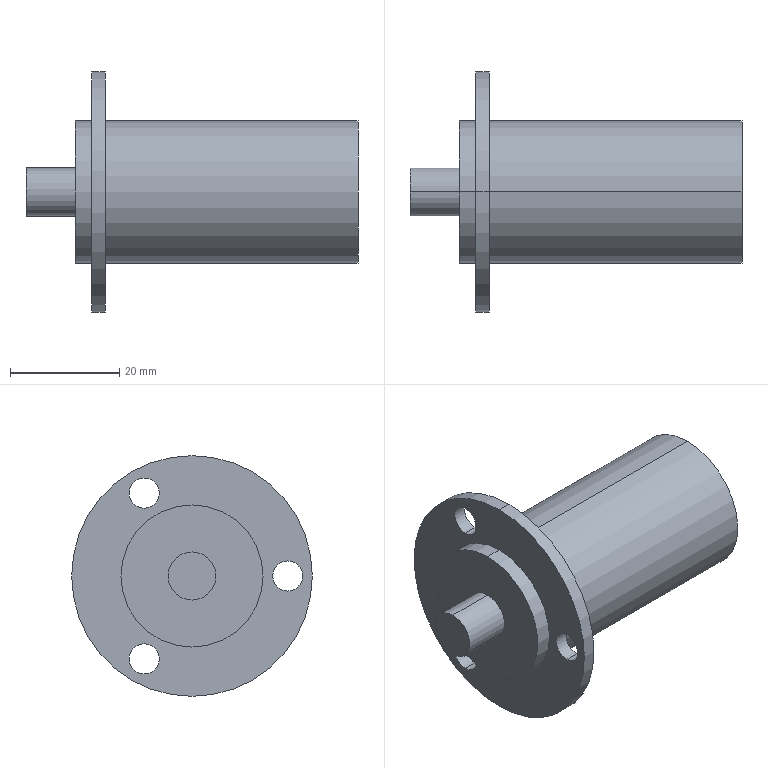Part | STEP file | SRC025-30 rotary joint_SUS304 | 1 solid | 19 faces | box 60.7 x 44 x 44 mm | volume 30292 mm3 | cylinder 14 | plane 5 | commonest cylinder face diameters 5.5 x6 26 x4 8.8 x2 44 x2
STEP:
#1=CARTESIAN_POINT('',(0.,0.,0.));
#2=DIRECTION('',(0.,0.,1.));
#3=DIRECTION('',(1.,0.,0.));
#4=AXIS2_PLACEMENT_3D('',#1,#2,#3);
#5=CARTESIAN_POINT('',(60.7,0.,13.));
#6=VERTEX_POINT('',#5);
#7=CARTESIAN_POINT('',(60.7,0.,-13.));
#8=VERTEX_POINT('',#7);
#9=CARTESIAN_POINT('',(60.7,0.,0.));
#10=DIRECTION('',(-1.,0.,0.));
#11=DIRECTION('',(0.,0.,1.));
#12=AXIS2_PLACEMENT_3D('',#9,#10,#11);
#13=CIRCLE('',#12,13.);
#14=CARTESIAN_POINT('',(60.7,0.,0.));
#15=DIRECTION('',(-1.,0.,0.));
#16=DIRECTION('',(0.,0.,1.));
#17=AXIS2_PLACEMENT_3D('',#14,#15,#16);
#18=CYLINDRICAL_SURFACE('',#17,13.);
#19=CARTESIAN_POINT('',(0.,0.));
#20=DIRECTION('',(1.,0.));
#21=VECTOR('',#20,1.);
#22=LINE('',#19,#21);
#23=(GEOMETRIC_REPRESENTATION_CONTEXT(2)PARAMETRIC_REPRESENTATION_CONTEXT()REPRESENTATION_CONTEXT('',''));
#24=DEFINITIONAL_REPRESENTATION('',(#22),#23);
#25=PCURVE('',#18,#24);
#26=CARTESIAN_POINT('',(60.7,0.,0.));
#27=DIRECTION('',(1.,0.,0.));
#28=DIRECTION('',(0.,0.,-1.));
#29=AXIS2_PLACEMENT_3D('',#26,#27,#28);
#30=PLANE('',#29);
#31=CARTESIAN_POINT('',(-13.,0.));
#32=CARTESIAN_POINT('',(-13.,22.517));
#33=CARTESIAN_POINT('',(6.5,11.258));
#34=CARTESIAN_POINT('',(26.,0.));
#35=CARTESIAN_POINT('',(6.5,-11.258));
#36=CARTESIAN_POINT('',(-13.,-22.517));
#37=CARTESIAN_POINT('',(-13.,0.));
#38=(BOUNDED_CURVE()B_SPLINE_CURVE(2,(#31,#32,#33,#34,#35,#36,#37),.UNSPECIFIED.,.T.,.F.)B_SPLINE_CURVE_WITH_KNOTS((1,2,2,2,2,1),(-2.094,0.,2.094,4.189,6.283,8.378),.UNSPECIFIED.)CURVE()GEOMETRIC_REPRESENTATION_ITEM()RATIONAL_B_SPLINE_CURVE((1.,0.5,1.,0.5,1.,0.5,1.))REPRESENTATION_ITEM(''));
#39=(GEOMETRIC_REPRESENTATION_CONTEXT(2)PARAMETRIC_REPRESENTATION_CONTEXT()REPRESENTATION_CONTEXT('',''));
#40=DEFINITIONAL_REPRESENTATION('',(#38),#39);
#41=PCURVE('',#30,#40);
#42=SURFACE_CURVE('',#13,(#25,#41),.PCURVE_S1.);
#43=EDGE_CURVE('',#6,#8,#42,.T.);
#44=ORIENTED_EDGE('',*,*,#43,.T.);
#45=CARTESIAN_POINT('',(14.5,0.,-13.));
#46=VERTEX_POINT('',#45);
#47=CARTESIAN_POINT('',(60.7,0.,-13.));
#48=DIRECTION('',(-1.,0.,0.));
#49=VECTOR('',#48,1.);
#50=LINE('',#47,#49);
#51=CARTESIAN_POINT('',(3.142,0.));
#52=DIRECTION('',(0.,1.));
#53=VECTOR('',#52,1.);
#54=LINE('',#51,#53);
#55=(GEOMETRIC_REPRESENTATION_CONTEXT(2)PARAMETRIC_REPRESENTATION_CONTEXT()REPRESENTATION_CONTEXT('',''));
#56=DEFINITIONAL_REPRESENTATION('',(#54),#55);
#57=PCURVE('',#18,#56);
#58=CARTESIAN_POINT('',(60.7,0.,0.));
#59=DIRECTION('',(-1.,0.,0.));
#60=DIRECTION('',(0.,0.,1.));
#61=AXIS2_PLACEMENT_3D('',#58,#59,#60);
#62=CYLINDRICAL_SURFACE('',#61,13.);
#63=CARTESIAN_POINT('',(3.142,0.));
#64=DIRECTION('',(0.,1.));
#65=VECTOR('',#64,1.);
#66=LINE('',#63,#65);
#67=(GEOMETRIC_REPRESENTATION_CONTEXT(2)PARAMETRIC_REPRESENTATION_CONTEXT()REPRESENTATION_CONTEXT('',''));
#68=DEFINITIONAL_REPRESENTATION('',(#66),#67);
#69=PCURVE('',#62,#68);
#70=SURFACE_CURVE('',#50,(#57,#69),.PCURVE_S1.);
#71=EDGE_CURVE('',#8,#46,#70,.T.);
#72=ORIENTED_EDGE('',*,*,#71,.T.);
#73=CARTESIAN_POINT('',(14.5,0.,13.));
#74=VERTEX_POINT('',#73);
#75=CARTESIAN_POINT('',(14.5,0.,0.));
#76=DIRECTION('',(1.,0.,0.));
#77=DIRECTION('',(0.,0.,1.));
#78=AXIS2_PLACEMENT_3D('',#75,#76,#77);
#79=CIRCLE('',#78,13.);
#80=CARTESIAN_POINT('',(6.283,46.2));
#81=DIRECTION('',(-1.,0.));
#82=VECTOR('',#81,1.);
#83=LINE('',#80,#82);
#84=(GEOMETRIC_REPRESENTATION_CONTEXT(2)PARAMETRIC_REPRESENTATION_CONTEXT()REPRESENTATION_CONTEXT('',''));
#85=DEFINITIONAL_REPRESENTATION('',(#83),#84);
#86=PCURVE('',#18,#85);
#87=CARTESIAN_POINT('',(14.5,0.,0.));
#88=DIRECTION('',(1.,0.,0.));
#89=DIRECTION('',(0.,0.,-1.));
#90=AXIS2_PLACEMENT_3D('',#87,#88,#89);
#91=PLANE('',#90);
#92=CARTESIAN_POINT('',(0.,0.));
#93=DIRECTION('',(-1.,0.));
#94=AXIS2_PLACEMENT_2D('',#92,#93);
#95=CIRCLE('',#94,13.);
#96=(GEOMETRIC_REPRESENTATION_CONTEXT(2)PARAMETRIC_REPRESENTATION_CONTEXT()REPRESENTATION_CONTEXT('',''));
#97=DEFINITIONAL_REPRESENTATION('',(#95),#96);
#98=PCURVE('',#91,#97);
#99=SURFACE_CURVE('',#79,(#86,#98),.PCURVE_S1.);
#100=EDGE_CURVE('',#46,#74,#99,.T.);
#101=ORIENTED_EDGE('',*,*,#100,.T.);
#102=CARTESIAN_POINT('',(60.7,0.,13.));
#103=DIRECTION('',(-1.,0.,0.));
#104=VECTOR('',#103,1.);
#105=LINE('',#102,#104);
#106=CARTESIAN_POINT('',(0.,0.));
#107=DIRECTION('',(0.,1.));
#108=VECTOR('',#107,1.);
#109=LINE('',#106,#108);
#110=(GEOMETRIC_REPRESENTATION_CONTEXT(2)PARAMETRIC_REPRESENTATION_CONTEXT()REPRESENTATION_CONTEXT('',''));
#111=DEFINITIONAL_REPRESENTATION('',(#109),#110);
#112=PCURVE('',#18,#111);
#113=CARTESIAN_POINT('',(6.283,0.));
#114=DIRECTION('',(0.,1.));
#115=VECTOR('',#114,1.);
#116=LINE('',#113,#115);
#117=(GEOMETRIC_REPRESENTATION_CONTEXT(2)PARAMETRIC_REPRESENTATION_CONTEXT()REPRESENTATION_CONTEXT('',''));
#118=DEFINITIONAL_REPRESENTATION('',(#116),#117);
#119=PCURVE('',#62,#118);
#120=SURFACE_CURVE('',#105,(#112,#119),.PCURVE_S1.);
#121=EDGE_CURVE('',#6,#74,#120,.T.);
#122=ORIENTED_EDGE('',*,*,#121,.F.);
#123=EDGE_LOOP('',(#44,#72,#101,#122));
#124=FACE_BOUND('',#123,.T.);
#125=ADVANCED_FACE('',(#124),#18,.T.);
#126=CARTESIAN_POINT('',(14.5,-17.5,2.75));
#127=VERTEX_POINT('',#126);
#128=CARTESIAN_POINT('',(12.,-17.5,2.75));
#129=VERTEX_POINT('',#128);
#130=CARTESIAN_POINT('',(58.2,-17.5,2.75));
#131=DIRECTION('',(-1.,0.,0.));
#132=VECTOR('',#131,1.);
#133=LINE('',#130,#132);
#134=CARTESIAN_POINT('',(58.2,-17.5,0.));
#135=DIRECTION('',(-1.,0.,0.));
#136=DIRECTION('',(0.,0.,1.));
#137=AXIS2_PLACEMENT_3D('',#134,#135,#136);
#138=CYLINDRICAL_SURFACE('',#137,2.75);
#139=CARTESIAN_POINT('',(6.283,0.));
#140=DIRECTION('',(0.,1.));
#141=VECTOR('',#140,1.);
#142=LINE('',#139,#141);
#143=(GEOMETRIC_REPRESENTATION_CONTEXT(2)PARAMETRIC_REPRESENTATION_CONTEXT()REPRESENTATION_CONTEXT('',''));
#144=DEFINITIONAL_REPRESENTATION('',(#142),#143);
#145=PCURVE('',#138,#144);
#146=CARTESIAN_POINT('',(58.2,-17.5,0.));
#147=DIRECTION('',(-1.,0.,0.));
#148=DIRECTION('',(0.,0.,1.));
#149=AXIS2_PLACEMENT_3D('',#146,#147,#148);
#150=CYLINDRICAL_SURFACE('',#149,2.75);
#151=CARTESIAN_POINT('',(0.,0.));
#152=DIRECTION('',(0.,1.));
#153=VECTOR('',#152,1.);
#154=LINE('',#151,#153);
#155=(GEOMETRIC_REPRESENTATION_CONTEXT(2)PARAMETRIC_REPRESENTATION_CONTEXT()REPRESENTATION_CONTEXT('',''));
#156=DEFINITIONAL_REPRESENTATION('',(#154),#155);
#157=PCURVE('',#150,#156);
#158=SURFACE_CURVE('',#133,(#145,#157),.PCURVE_S1.);
#159=EDGE_CURVE('',#127,#129,#158,.T.);
#160=ORIENTED_EDGE('',*,*,#159,.T.);
#161=CARTESIAN_POINT('',(12.,-17.5,-2.75));
#162=VERTEX_POINT('',#161);
#163=CARTESIAN_POINT('',(12.,-17.5,0.));
#164=DIRECTION('',(1.,0.,0.));
#165=DIRECTION('',(0.,0.,1.));
#166=AXIS2_PLACEMENT_3D('',#163,#164,#165);
#167=CIRCLE('',#166,2.75);
#168=CARTESIAN_POINT('',(6.283,46.2));
#169=DIRECTION('',(-1.,0.));
#170=VECTOR('',#169,1.);
#171=LINE('',#168,#170);
#172=(GEOMETRIC_REPRESENTATION_CONTEXT(2)PARAMETRIC_REPRESENTATION_CONTEXT()REPRESENTATION_CONTEXT('',''));
#173=DEFINITIONAL_REPRESENTATION('',(#171),#172);
#174=PCURVE('',#138,#173);
#175=CARTESIAN_POINT('',(12.,0.,0.));
#176=DIRECTION('',(1.,0.,0.));
#177=DIRECTION('',(0.,0.,-1.));
#178=AXIS2_PLACEMENT_3D('',#175,#176,#177);
#179=PLANE('',#178);
#180=CARTESIAN_POINT('',(0.,-17.5));
#181=DIRECTION('',(-1.,0.));
#182=AXIS2_PLACEMENT_2D('',#180,#181);
#183=CIRCLE('',#182,2.75);
#184=(GEOMETRIC_REPRESENTATION_CONTEXT(2)PARAMETRIC_REPRESENTATION_CONTEXT()REPRESENTATION_CONTEXT('',''));
#185=DEFINITIONAL_REPRESENTATION('',(#183),#184);
#186=PCURVE('',#179,#185);
#187=SURFACE_CURVE('',#167,(#174,#186),.PCURVE_S1.);
#188=EDGE_CURVE('',#129,#162,#187,.T.);
#189=ORIENTED_EDGE('',*,*,#188,.T.);
#190=CARTESIAN_POINT('',(14.5,-17.5,-2.75));
#191=VERTEX_POINT('',#190);
#192=CARTESIAN_POINT('',(58.2,-17.5,-2.75));
#193=DIRECTION('',(-1.,0.,0.));
#194=VECTOR('',#193,1.);
#195=LINE('',#192,#194);
#196=CARTESIAN_POINT('',(3.142,0.));
#197=DIRECTION('',(0.,1.));
#198=VECTOR('',#197,1.);
#199=LINE('',#196,#198);
#200=(GEOMETRIC_REPRESENTATION_CONTEXT(2)PARAMETRIC_REPRESENTATION_CONTEXT()REPRESENTATION_CONTEXT('',''));
#201=DEFINITIONAL_REPRESENTATION('',(#199),#200);
#202=PCURVE('',#138,#201);
#203=CARTESIAN_POINT('',(3.142,0.));
#204=DIRECTION('',(0.,1.));
#205=VECTOR('',#204,1.);
#206=LINE('',#203,#205);
#207=(GEOMETRIC_REPRESENTATION_CONTEXT(2)PARAMETRIC_REPRESENTATION_CONTEXT()REPRESENTATION_CONTEXT('',''));
#208=DEFINITIONAL_REPRESENTATION('',(#206),#207);
#209=PCURVE('',#150,#208);
#210=SURFACE_CURVE('',#195,(#202,#209),.PCURVE_S1.);
#211=EDGE_CURVE('',#191,#162,#210,.T.);
#212=ORIENTED_EDGE('',*,*,#211,.F.);
#213=CARTESIAN_POINT('',(14.5,-17.5,0.));
#214=DIRECTION('',(-1.,0.,0.));
#215=DIRECTION('',(0.,0.,1.));
#216=AXIS2_PLACEMENT_3D('',#213,#214,#215);
#217=CIRCLE('',#216,2.75);
#218=CARTESIAN_POINT('',(0.,43.7));
#219=DIRECTION('',(1.,0.));
#220=VECTOR('',#219,1.);
#221=LINE('',#218,#220);
#222=(GEOMETRIC_REPRESENTATION_CONTEXT(2)PARAMETRIC_REPRESENTATION_CONTEXT()REPRESENTATION_CONTEXT('',''));
#223=DEFINITIONAL_REPRESENTATION('',(#221),#222);
#224=PCURVE('',#138,#223);
#225=CARTESIAN_POINT('',(-2.75,-17.5));
#226=CARTESIAN_POINT('',(-2.75,-12.737));
#227=CARTESIAN_POINT('',(1.375,-15.118));
#228=CARTESIAN_POINT('',(5.5,-17.5));
#229=CARTESIAN_POINT('',(1.375,-19.882));
#230=CARTESIAN_POINT('',(-2.75,-22.263));
#231=CARTESIAN_POINT('',(-2.75,-17.5));
#232=(BOUNDED_CURVE()B_SPLINE_CURVE(2,(#225,#226,#227,#228,#229,#230,#231),.UNSPECIFIED.,.T.,.F.)B_SPLINE_CURVE_WITH_KNOTS((1,2,2,2,2,1),(-2.094,0.,2.094,4.189,6.283,8.378),.UNSPECIFIED.)CURVE()GEOMETRIC_REPRESENTATION_ITEM()RATIONAL_B_SPLINE_CURVE((1.,0.5,1.,0.5,1.,0.5,1.))REPRESENTATION_ITEM(''));
#233=(GEOMETRIC_REPRESENTATION_CONTEXT(2)PARAMETRIC_REPRESENTATION_CONTEXT()REPRESENTATION_CONTEXT('',''));
#234=DEFINITIONAL_REPRESENTATION('',(#232),#233);
#235=PCURVE('',#91,#234);
#236=SURFACE_CURVE('',#217,(#224,#235),.PCURVE_S1.);
#237=EDGE_CURVE('',#191,#127,#236,.T.);
#238=ORIENTED_EDGE('',*,*,#237,.T.);
#239=EDGE_LOOP('',(#160,#189,#212,#238));
#240=FACE_BOUND('',#239,.F.);
#241=ADVANCED_FACE('',(#240),#138,.F.);
#242=CARTESIAN_POINT('',(14.5,8.75,-12.405));
#243=VERTEX_POINT('',#242);
#244=CARTESIAN_POINT('',(12.,8.75,-12.405));
#245=VERTEX_POINT('',#244);
#246=CARTESIAN_POINT('',(58.2,8.75,-12.405));
#247=DIRECTION('',(-1.,0.,0.));
#248=VECTOR('',#247,1.);
#249=LINE('',#246,#248);
#250=CARTESIAN_POINT('',(58.2,8.75,-15.155));
#251=DIRECTION('',(-1.,0.,0.));
#252=DIRECTION('',(0.,0.,1.));
#253=AXIS2_PLACEMENT_3D('',#250,#251,#252);
#254=CYLINDRICAL_SURFACE('',#253,2.75);
#255=CARTESIAN_POINT('',(6.283,0.));
#256=DIRECTION('',(0.,1.));
#257=VECTOR('',#256,1.);
#258=LINE('',#255,#257);
#259=(GEOMETRIC_REPRESENTATION_CONTEXT(2)PARAMETRIC_REPRESENTATION_CONTEXT()REPRESENTATION_CONTEXT('',''));
#260=DEFINITIONAL_REPRESENTATION('',(#258),#259);
#261=PCURVE('',#254,#260);
#262=CARTESIAN_POINT('',(58.2,8.75,-15.155));
#263=DIRECTION('',(-1.,0.,0.));
#264=DIRECTION('',(0.,0.,1.));
#265=AXIS2_PLACEMENT_3D('',#262,#263,#264);
#266=CYLINDRICAL_SURFACE('',#265,2.75);
#267=CARTESIAN_POINT('',(0.,0.));
#268=DIRECTION('',(0.,1.));
#269=VECTOR('',#268,1.);
#270=LINE('',#267,#269);
#271=(GEOMETRIC_REPRESENTATION_CONTEXT(2)PARAMETRIC_REPRESENTATION_CONTEXT()REPRESENTATION_CONTEXT('',''));
#272=DEFINITIONAL_REPRESENTATION('',(#270),#271);
#273=PCURVE('',#266,#272);
#274=SURFACE_CURVE('',#249,(#261,#273),.PCURVE_S1.);
#275=EDGE_CURVE('',#243,#245,#274,.T.);
#276=ORIENTED_EDGE('',*,*,#275,.T.);
#277=CARTESIAN_POINT('',(12.,8.75,-17.905));
#278=VERTEX_POINT('',#277);
#279=CARTESIAN_POINT('',(12.,8.75,-15.155));
#280=DIRECTION('',(1.,0.,0.));
#281=DIRECTION('',(0.,0.,1.));
#282=AXIS2_PLACEMENT_3D('',#279,#280,#281);
#283=CIRCLE('',#282,2.75);
#284=CARTESIAN_POINT('',(6.283,46.2));
#285=DIRECTION('',(-1.,0.));
#286=VECTOR('',#285,1.);
#287=LINE('',#284,#286);
#288=(GEOMETRIC_REPRESENTATION_CONTEXT(2)PARAMETRIC_REPRESENTATION_CONTEXT()REPRESENTATION_CONTEXT('',''));
#289=DEFINITIONAL_REPRESENTATION('',(#287),#288);
#290=PCURVE('',#254,#289);
#291=CARTESIAN_POINT('',(15.155,8.75));
#292=DIRECTION('',(-1.,0.));
#293=AXIS2_PLACEMENT_2D('',#291,#292);
#294=CIRCLE('',#293,2.75);
#295=(GEOMETRIC_REPRESENTATION_CONTEXT(2)PARAMETRIC_REPRESENTATION_CONTEXT()REPRESENTATION_CONTEXT('',''));
#296=DEFINITIONAL_REPRESENTATION('',(#294),#295);
#297=PCURVE('',#179,#296);
#298=SURFACE_CURVE('',#283,(#290,#297),.PCURVE_S1.);
#299=EDGE_CURVE('',#245,#278,#298,.T.);
#300=ORIENTED_EDGE('',*,*,#299,.T.);
#301=CARTESIAN_POINT('',(14.5,8.75,-17.905));
#302=VERTEX_POINT('',#301);
#303=CARTESIAN_POINT('',(58.2,8.75,-17.905));
#304=DIRECTION('',(-1.,0.,0.));
#305=VECTOR('',#304,1.);
#306=LINE('',#303,#305);
#307=CARTESIAN_POINT('',(3.142,0.));
#308=DIRECTION('',(0.,1.));
#309=VECTOR('',#308,1.);
#310=LINE('',#307,#309);
#311=(GEOMETRIC_REPRESENTATION_CONTEXT(2)PARAMETRIC_REPRESENTATION_CONTEXT()REPRESENTATION_CONTEXT('',''));
#312=DEFINITIONAL_REPRESENTATION('',(#310),#311);
#313=PCURVE('',#254,#312);
#314=CARTESIAN_POINT('',(3.142,0.));
#315=DIRECTION('',(0.,1.));
#316=VECTOR('',#315,1.);
#317=LINE('',#314,#316);
#318=(GEOMETRIC_REPRESENTATION_CONTEXT(2)PARAMETRIC_REPRESENTATION_CONTEXT()REPRESENTATION_CONTEXT('',''));
#319=DEFINITIONAL_REPRESENTATION('',(#317),#318);
#320=PCURVE('',#266,#319);
#321=SURFACE_CURVE('',#306,(#313,#320),.PCURVE_S1.);
#322=EDGE_CURVE('',#302,#278,#321,.T.);
#323=ORIENTED_EDGE('',*,*,#322,.F.);
#324=CARTESIAN_POINT('',(14.5,8.75,-15.155));
#325=DIRECTION('',(-1.,0.,0.));
#326=DIRECTION('',(0.,0.,1.));
#327=AXIS2_PLACEMENT_3D('',#324,#325,#326);
#328=CIRCLE('',#327,2.75);
#329=CARTESIAN_POINT('',(0.,43.7));
#330=DIRECTION('',(1.,0.));
#331=VECTOR('',#330,1.);
#332=LINE('',#329,#331);
#333=(GEOMETRIC_REPRESENTATION_CONTEXT(2)PARAMETRIC_REPRESENTATION_CONTEXT()REPRESENTATION_CONTEXT('',''));
#334=DEFINITIONAL_REPRESENTATION('',(#332),#333);
#335=PCURVE('',#254,#334);
#336=CARTESIAN_POINT('',(12.405,8.75));
#337=CARTESIAN_POINT('',(12.405,13.513));
#338=CARTESIAN_POINT('',(16.53,11.132));
#339=CARTESIAN_POINT('',(20.655,8.75));
#340=CARTESIAN_POINT('',(16.53,6.368));
#341=CARTESIAN_POINT('',(12.405,3.987));
#342=CARTESIAN_POINT('',(12.405,8.75));
#343=(BOUNDED_CURVE()B_SPLINE_CURVE(2,(#336,#337,#338,#339,#340,#341,#342),.UNSPECIFIED.,.T.,.F.)B_SPLINE_CURVE_WITH_KNOTS((1,2,2,2,2,1),(-2.094,0.,2.094,4.189,6.283,8.378),.UNSPECIFIED.)CURVE()GEOMETRIC_REPRESENTATION_ITEM()RATIONAL_B_SPLINE_CURVE((1.,0.5,1.,0.5,1.,0.5,1.))REPRESENTATION_ITEM(''));
#344=(GEOMETRIC_REPRESENTATION_CONTEXT(2)PARAMETRIC_REPRESENTATION_CONTEXT()REPRESENTATION_CONTEXT('',''));
#345=DEFINITIONAL_REPRESENTATION('',(#343),#344);
#346=PCURVE('',#91,#345);
#347=SURFACE_CURVE('',#328,(#335,#346),.PCURVE_S1.);
#348=EDGE_CURVE('',#302,#243,#347,.T.);
#349=ORIENTED_EDGE('',*,*,#348,.T.);
#350=EDGE_LOOP('',(#276,#300,#323,#349));
#351=FACE_BOUND('',#350,.F.);
#352=ADVANCED_FACE('',(#351),#254,.F.);
#353=CARTESIAN_POINT('',(14.5,8.75,17.905));
#354=VERTEX_POINT('',#353);
#355=CARTESIAN_POINT('',(12.,8.75,17.905));
#356=VERTEX_POINT('',#355);
#357=CARTESIAN_POINT('',(58.2,8.75,17.905));
#358=DIRECTION('',(-1.,0.,0.));
#359=VECTOR('',#358,1.);
#360=LINE('',#357,#359);
#361=CARTESIAN_POINT('',(58.2,8.75,15.155));
#362=DIRECTION('',(-1.,0.,0.));
#363=DIRECTION('',(0.,0.,1.));
#364=AXIS2_PLACEMENT_3D('',#361,#362,#363);
#365=CYLINDRICAL_SURFACE('',#364,2.75);
#366=CARTESIAN_POINT('',(6.283,0.));
#367=DIRECTION('',(0.,1.));
#368=VECTOR('',#367,1.);
#369=LINE('',#366,#368);
#370=(GEOMETRIC_REPRESENTATION_CONTEXT(2)PARAMETRIC_REPRESENTATION_CONTEXT()REPRESENTATION_CONTEXT('',''));
#371=DEFINITIONAL_REPRESENTATION('',(#369),#370);
#372=PCURVE('',#365,#371);
#373=CARTESIAN_POINT('',(58.2,8.75,15.155));
#374=DIRECTION('',(-1.,0.,0.));
#375=DIRECTION('',(0.,0.,1.));
#376=AXIS2_PLACEMENT_3D('',#373,#374,#375);
#377=CYLINDRICAL_SURFACE('',#376,2.75);
#378=CARTESIAN_POINT('',(0.,0.));
#379=DIRECTION('',(0.,1.));
#380=VECTOR('',#379,1.);
#381=LINE('',#378,#380);
#382=(GEOMETRIC_REPRESENTATION_CONTEXT(2)PARAMETRIC_REPRESENTATION_CONTEXT()REPRESENTATION_CONTEXT('',''));
#383=DEFINITIONAL_REPRESENTATION('',(#381),#382);
#384=PCURVE('',#377,#383);
#385=SURFACE_CURVE('',#360,(#372,#384),.PCURVE_S1.);
#386=EDGE_CURVE('',#354,#356,#385,.T.);
#387=ORIENTED_EDGE('',*,*,#386,.T.);
#388=CARTESIAN_POINT('',(12.,8.75,12.405));
#389=VERTEX_POINT('',#388);
#390=CARTESIAN_POINT('',(12.,8.75,15.155));
#391=DIRECTION('',(1.,0.,0.));
#392=DIRECTION('',(0.,0.,1.));
#393=AXIS2_PLACEMENT_3D('',#390,#391,#392);
#394=CIRCLE('',#393,2.75);
#395=CARTESIAN_POINT('',(6.283,46.2));
#396=DIRECTION('',(-1.,0.));
#397=VECTOR('',#396,1.);
#398=LINE('',#395,#397);
#399=(GEOMETRIC_REPRESENTATION_CONTEXT(2)PARAMETRIC_REPRESENTATION_CONTEXT()REPRESENTATION_CONTEXT('',''));
#400=DEFINITIONAL_REPRESENTATION('',(#398),#399);
#401=PCURVE('',#365,#400);
#402=CARTESIAN_POINT('',(-15.155,8.75));
#403=DIRECTION('',(-1.,0.));
#404=AXIS2_PLACEMENT_2D('',#402,#403);
#405=CIRCLE('',#404,2.75);
#406=(GEOMETRIC_REPRESENTATION_CONTEXT(2)PARAMETRIC_REPRESENTATION_CONTEXT()REPRESENTATION_CONTEXT('',''));
#407=DEFINITIONAL_REPRESENTATION('',(#405),#406);
#408=PCURVE('',#179,#407);
#409=SURFACE_CURVE('',#394,(#401,#408),.PCURVE_S1.);
#410=EDGE_CURVE('',#356,#389,#409,.T.);
#411=ORIENTED_EDGE('',*,*,#410,.T.);
#412=CARTESIAN_POINT('',(14.5,8.75,12.405));
#413=VERTEX_POINT('',#412);
#414=CARTESIAN_POINT('',(58.2,8.75,12.405));
#415=DIRECTION('',(-1.,0.,0.));
#416=VECTOR('',#415,1.);
#417=LINE('',#414,#416);
#418=CARTESIAN_POINT('',(3.142,0.));
#419=DIRECTION('',(0.,1.));
#420=VECTOR('',#419,1.);
#421=LINE('',#418,#420);
#422=(GEOMETRIC_REPRESENTATION_CONTEXT(2)PARAMETRIC_REPRESENTATION_CONTEXT()REPRESENTATION_CONTEXT('',''));
#423=DEFINITIONAL_REPRESENTATION('',(#421),#422);
#424=PCURVE('',#365,#423);
#425=CARTESIAN_POINT('',(3.142,0.));
#426=DIRECTION('',(0.,1.));
#427=VECTOR('',#426,1.);
#428=LINE('',#425,#427);
#429=(GEOMETRIC_REPRESENTATION_CONTEXT(2)PARAMETRIC_REPRESENTATION_CONTEXT()REPRESENTATION_CONTEXT('',''));
#430=DEFINITIONAL_REPRESENTATION('',(#428),#429);
#431=PCURVE('',#377,#430);
#432=SURFACE_CURVE('',#417,(#424,#431),.PCURVE_S1.);
#433=EDGE_CURVE('',#413,#389,#432,.T.);
#434=ORIENTED_EDGE('',*,*,#433,.F.);
#435=CARTESIAN_POINT('',(14.5,8.75,15.155));
#436=DIRECTION('',(-1.,0.,0.));
#437=DIRECTION('',(0.,0.,1.));
#438=AXIS2_PLACEMENT_3D('',#435,#436,#437);
#439=CIRCLE('',#438,2.75);
#440=CARTESIAN_POINT('',(0.,43.7));
#441=DIRECTION('',(1.,0.));
#442=VECTOR('',#441,1.);
#443=LINE('',#440,#442);
#444=(GEOMETRIC_REPRESENTATION_CONTEXT(2)PARAMETRIC_REPRESENTATION_CONTEXT()REPRESENTATION_CONTEXT('',''));
#445=DEFINITIONAL_REPRESENTATION('',(#443),#444);
#446=PCURVE('',#365,#445);
#447=CARTESIAN_POINT('',(-17.905,8.75));
#448=CARTESIAN_POINT('',(-17.905,13.513));
#449=CARTESIAN_POINT('',(-13.78,11.132));
#450=CARTESIAN_POINT('',(-9.655,8.75));
#451=CARTESIAN_POINT('',(-13.78,6.368));
#452=CARTESIAN_POINT('',(-17.905,3.987));
#453=CARTESIAN_POINT('',(-17.905,8.75));
#454=(BOUNDED_CURVE()B_SPLINE_CURVE(2,(#447,#448,#449,#450,#451,#452,#453),.UNSPECIFIED.,.T.,.F.)B_SPLINE_CURVE_WITH_KNOTS((1,2,2,2,2,1),(-2.094,0.,2.094,4.189,6.283,8.378),.UNSPECIFIED.)CURVE()GEOMETRIC_REPRESENTATION_ITEM()RATIONAL_B_SPLINE_CURVE((1.,0.5,1.,0.5,1.,0.5,1.))REPRESENTATION_ITEM(''));
#455=(GEOMETRIC_REPRESENTATION_CONTEXT(2)PARAMETRIC_REPRESENTATION_CONTEXT()REPRESENTATION_CONTEXT('',''));
#456=DEFINITIONAL_REPRESENTATION('',(#454),#455);
#457=PCURVE('',#91,#456);
#458=SURFACE_CURVE('',#439,(#446,#457),.PCURVE_S1.);
#459=EDGE_CURVE('',#413,#354,#458,.T.);
#460=ORIENTED_EDGE('',*,*,#459,.T.);
#461=EDGE_LOOP('',(#387,#411,#434,#460));
#462=FACE_BOUND('',#461,.F.);
#463=ADVANCED_FACE('',(#462),#365,.F.);
#464=CARTESIAN_POINT('',(14.5,0.,-22.));
#465=VERTEX_POINT('',#464);
#466=CARTESIAN_POINT('',(14.5,0.,22.));
#467=VERTEX_POINT('',#466);
#468=CARTESIAN_POINT('',(14.5,0.,0.));
#469=DIRECTION('',(1.,0.,0.));
#470=DIRECTION('',(0.,0.,1.));
#471=AXIS2_PLACEMENT_3D('',#468,#469,#470);
#472=CIRCLE('',#471,22.);
#473=CARTESIAN_POINT('',(14.5,0.,0.));
#474=DIRECTION('',(-1.,0.,0.));
#475=DIRECTION('',(0.,0.,1.));
#476=AXIS2_PLACEMENT_3D('',#473,#474,#475);
#477=CYLINDRICAL_SURFACE('',#476,22.);
#478=CARTESIAN_POINT('',(6.283,0.));
#479=DIRECTION('',(-1.,0.));
#480=VECTOR('',#479,1.);
#481=LINE('',#478,#480);
#482=(GEOMETRIC_REPRESENTATION_CONTEXT(2)PARAMETRIC_REPRESENTATION_CONTEXT()REPRESENTATION_CONTEXT('',''));
#483=DEFINITIONAL_REPRESENTATION('',(#481),#482);
#484=PCURVE('',#477,#483);
#485=CARTESIAN_POINT('',(0.,0.));
#486=DIRECTION('',(-1.,0.));
#487=AXIS2_PLACEMENT_2D('',#485,#486);
#488=CIRCLE('',#487,22.);
#489=(GEOMETRIC_REPRESENTATION_CONTEXT(2)PARAMETRIC_REPRESENTATION_CONTEXT()REPRESENTATION_CONTEXT('',''));
#490=DEFINITIONAL_REPRESENTATION('',(#488),#489);
#491=PCURVE('',#91,#490);
#492=SURFACE_CURVE('',#472,(#484,#491),.PCURVE_S1.);
#493=EDGE_CURVE('',#465,#467,#492,.T.);
#494=ORIENTED_EDGE('',*,*,#493,.F.);
#495=CARTESIAN_POINT('',(12.,0.,-22.));
#496=VERTEX_POINT('',#495);
#497=CARTESIAN_POINT('',(14.5,0.,-22.));
#498=DIRECTION('',(-1.,0.,0.));
#499=VECTOR('',#498,1.);
#500=LINE('',#497,#499);
#501=CARTESIAN_POINT('',(3.142,0.));
#502=DIRECTION('',(0.,1.));
#503=VECTOR('',#502,1.);
#504=LINE('',#501,#503);
#505=(GEOMETRIC_REPRESENTATION_CONTEXT(2)PARAMETRIC_REPRESENTATION_CONTEXT()REPRESENTATION_CONTEXT('',''));
#506=DEFINITIONAL_REPRESENTATION('',(#504),#505);
#507=PCURVE('',#477,#506);
#508=CARTESIAN_POINT('',(14.5,0.,0.));
#509=DIRECTION('',(-1.,0.,0.));
#510=DIRECTION('',(0.,0.,1.));
#511=AXIS2_PLACEMENT_3D('',#508,#509,#510);
#512=CYLINDRICAL_SURFACE('',#511,22.);
#513=CARTESIAN_POINT('',(3.142,0.));
#514=DIRECTION('',(0.,1.));
#515=VECTOR('',#514,1.);
#516=LINE('',#513,#515);
#517=(GEOMETRIC_REPRESENTATION_CONTEXT(2)PARAMETRIC_REPRESENTATION_CONTEXT()REPRESENTATION_CONTEXT('',''));
#518=DEFINITIONAL_REPRESENTATION('',(#516),#517);
#519=PCURVE('',#512,#518);
#520=SURFACE_CURVE('',#500,(#507,#519),.PCURVE_S1.);
#521=EDGE_CURVE('',#465,#496,#520,.T.);
#522=ORIENTED_EDGE('',*,*,#521,.T.);
#523=CARTESIAN_POINT('',(12.,0.,22.));
#524=VERTEX_POINT('',#523);
#525=CARTESIAN_POINT('',(12.,0.,0.));
#526=DIRECTION('',(1.,0.,0.));
#527=DIRECTION('',(0.,0.,1.));
#528=AXIS2_PLACEMENT_3D('',#525,#526,#527);
#529=CIRCLE('',#528,22.);
#530=CARTESIAN_POINT('',(6.283,2.5));
#531=DIRECTION('',(-1.,0.));
#532=VECTOR('',#531,1.);
#533=LINE('',#530,#532);
#534=(GEOMETRIC_REPRESENTATION_CONTEXT(2)PARAMETRIC_REPRESENTATION_CONTEXT()REPRESENTATION_CONTEXT('',''));
#535=DEFINITIONAL_REPRESENTATION('',(#533),#534);
#536=PCURVE('',#477,#535);
#537=CARTESIAN_POINT('',(0.,0.));
#538=DIRECTION('',(-1.,0.));
#539=AXIS2_PLACEMENT_2D('',#537,#538);
#540=CIRCLE('',#539,22.);
#541=(GEOMETRIC_REPRESENTATION_CONTEXT(2)PARAMETRIC_REPRESENTATION_CONTEXT()REPRESENTATION_CONTEXT('',''));
#542=DEFINITIONAL_REPRESENTATION('',(#540),#541);
#543=PCURVE('',#179,#542);
#544=SURFACE_CURVE('',#529,(#536,#543),.PCURVE_S1.);
#545=EDGE_CURVE('',#496,#524,#544,.T.);
#546=ORIENTED_EDGE('',*,*,#545,.T.);
#547=CARTESIAN_POINT('',(14.5,0.,22.));
#548=DIRECTION('',(-1.,0.,0.));
#549=VECTOR('',#548,1.);
#550=LINE('',#547,#549);
#551=CARTESIAN_POINT('',(0.,0.));
#552=DIRECTION('',(0.,1.));
#553=VECTOR('',#552,1.);
#554=LINE('',#551,#553);
#555=(GEOMETRIC_REPRESENTATION_CONTEXT(2)PARAMETRIC_REPRESENTATION_CONTEXT()REPRESENTATION_CONTEXT('',''));
#556=DEFINITIONAL_REPRESENTATION('',(#554),#555);
#557=PCURVE('',#477,#556);
#558=CARTESIAN_POINT('',(6.283,0.));
#559=DIRECTION('',(0.,1.));
#560=VECTOR('',#559,1.);
#561=LINE('',#558,#560);
#562=(GEOMETRIC_REPRESENTATION_CONTEXT(2)PARAMETRIC_REPRESENTATION_CONTEXT()REPRESENTATION_CONTEXT('',''));
#563=DEFINITIONAL_REPRESENTATION('',(#561),#562);
#564=PCURVE('',#512,#563);
#565=SURFACE_CURVE('',#550,(#557,#564),.PCURVE_S1.);
#566=EDGE_CURVE('',#467,#524,#565,.T.);
#567=ORIENTED_EDGE('',*,*,#566,.F.);
#568=EDGE_LOOP('',(#494,#522,#546,#567));
#569=FACE_BOUND('',#568,.T.);
#570=ADVANCED_FACE('',(#569),#477,.T.);
#571=CARTESIAN_POINT('',(12.,0.,13.));
#572=VERTEX_POINT('',#571);
#573=CARTESIAN_POINT('',(12.,0.,-13.));
#574=VERTEX_POINT('',#573);
#575=CARTESIAN_POINT('',(12.,0.,0.));
#576=DIRECTION('',(-1.,0.,0.));
#577=DIRECTION('',(0.,0.,1.));
#578=AXIS2_PLACEMENT_3D('',#575,#576,#577);
#579=CIRCLE('',#578,13.);
#580=CARTESIAN_POINT('',(12.,0.,0.));
#581=DIRECTION('',(-1.,0.,0.));
#582=DIRECTION('',(0.,0.,1.));
#583=AXIS2_PLACEMENT_3D('',#580,#581,#582);
#584=CYLINDRICAL_SURFACE('',#583,13.);
#585=CARTESIAN_POINT('',(0.,0.));
#586=DIRECTION('',(1.,0.));
#587=VECTOR('',#586,1.);
#588=LINE('',#585,#587);
#589=(GEOMETRIC_REPRESENTATION_CONTEXT(2)PARAMETRIC_REPRESENTATION_CONTEXT()REPRESENTATION_CONTEXT('',''));
#590=DEFINITIONAL_REPRESENTATION('',(#588),#589);
#591=PCURVE('',#584,#590);
#592=CARTESIAN_POINT('',(-13.,0.));
#593=CARTESIAN_POINT('',(-13.,22.517));
#594=CARTESIAN_POINT('',(6.5,11.258));
#595=CARTESIAN_POINT('',(26.,0.));
#596=CARTESIAN_POINT('',(6.5,-11.258));
#597=CARTESIAN_POINT('',(-13.,-22.517));
#598=CARTESIAN_POINT('',(-13.,0.));
#599=(BOUNDED_CURVE()B_SPLINE_CURVE(2,(#592,#593,#594,#595,#596,#597,#598),.UNSPECIFIED.,.T.,.F.)B_SPLINE_CURVE_WITH_KNOTS((1,2,2,2,2,1),(-2.094,0.,2.094,4.189,6.283,8.378),.UNSPECIFIED.)CURVE()GEOMETRIC_REPRESENTATION_ITEM()RATIONAL_B_SPLINE_CURVE((1.,0.5,1.,0.5,1.,0.5,1.))REPRESENTATION_ITEM(''));
#600=(GEOMETRIC_REPRESENTATION_CONTEXT(2)PARAMETRIC_REPRESENTATION_CONTEXT()REPRESENTATION_CONTEXT('',''));
#601=DEFINITIONAL_REPRESENTATION('',(#599),#600);
#602=PCURVE('',#179,#601);
#603=SURFACE_CURVE('',#579,(#591,#602),.PCURVE_S1.);
#604=EDGE_CURVE('',#572,#574,#603,.T.);
#605=ORIENTED_EDGE('',*,*,#604,.T.);
#606=CARTESIAN_POINT('',(9.,0.,-13.));
#607=VERTEX_POINT('',#606);
#608=CARTESIAN_POINT('',(12.,0.,-13.));
#609=DIRECTION('',(-1.,0.,0.));
#610=VECTOR('',#609,1.);
#611=LINE('',#608,#610);
#612=CARTESIAN_POINT('',(3.142,0.));
#613=DIRECTION('',(0.,1.));
#614=VECTOR('',#613,1.);
#615=LINE('',#612,#614);
#616=(GEOMETRIC_REPRESENTATION_CONTEXT(2)PARAMETRIC_REPRESENTATION_CONTEXT()REPRESENTATION_CONTEXT('',''));
#617=DEFINITIONAL_REPRESENTATION('',(#615),#616);
#618=PCURVE('',#584,#617);
#619=CARTESIAN_POINT('',(12.,0.,0.));
#620=DIRECTION('',(-1.,0.,0.));
#621=DIRECTION('',(0.,0.,1.));
#622=AXIS2_PLACEMENT_3D('',#619,#620,#621);
#623=CYLINDRICAL_SURFACE('',#622,13.);
#624=CARTESIAN_POINT('',(3.142,0.));
#625=DIRECTION('',(0.,1.));
#626=VECTOR('',#625,1.);
#627=LINE('',#624,#626);
#628=(GEOMETRIC_REPRESENTATION_CONTEXT(2)PARAMETRIC_REPRESENTATION_CONTEXT()REPRESENTATION_CONTEXT('',''));
#629=DEFINITIONAL_REPRESENTATION('',(#627),#628);
#630=PCURVE('',#623,#629);
#631=SURFACE_CURVE('',#611,(#618,#630),.PCURVE_S1.);
#632=EDGE_CURVE('',#574,#607,#631,.T.);
#633=ORIENTED_EDGE('',*,*,#632,.T.);
#634=CARTESIAN_POINT('',(9.,0.,13.));
#635=VERTEX_POINT('',#634);
#636=CARTESIAN_POINT('',(9.,0.,0.));
#637=DIRECTION('',(1.,0.,0.));
#638=DIRECTION('',(0.,0.,1.));
#639=AXIS2_PLACEMENT_3D('',#636,#637,#638);
#640=CIRCLE('',#639,13.);
#641=CARTESIAN_POINT('',(6.283,3.));
#642=DIRECTION('',(-1.,0.));
#643=VECTOR('',#642,1.);
#644=LINE('',#641,#643);
#645=(GEOMETRIC_REPRESENTATION_CONTEXT(2)PARAMETRIC_REPRESENTATION_CONTEXT()REPRESENTATION_CONTEXT('',''));
#646=DEFINITIONAL_REPRESENTATION('',(#644),#645);
#647=PCURVE('',#584,#646);
#648=CARTESIAN_POINT('',(9.,0.,0.));
#649=DIRECTION('',(1.,0.,0.));
#650=DIRECTION('',(0.,0.,-1.));
#651=AXIS2_PLACEMENT_3D('',#648,#649,#650);
#652=PLANE('',#651);
#653=CARTESIAN_POINT('',(0.,0.));
#654=DIRECTION('',(-1.,0.));
#655=AXIS2_PLACEMENT_2D('',#653,#654);
#656=CIRCLE('',#655,13.);
#657=(GEOMETRIC_REPRESENTATION_CONTEXT(2)PARAMETRIC_REPRESENTATION_CONTEXT()REPRESENTATION_CONTEXT('',''));
#658=DEFINITIONAL_REPRESENTATION('',(#656),#657);
#659=PCURVE('',#652,#658);
#660=SURFACE_CURVE('',#640,(#647,#659),.PCURVE_S1.);
#661=EDGE_CURVE('',#607,#635,#660,.T.);
#662=ORIENTED_EDGE('',*,*,#661,.T.);
#663=CARTESIAN_POINT('',(12.,0.,13.));
#664=DIRECTION('',(-1.,0.,0.));
#665=VECTOR('',#664,1.);
#666=LINE('',#663,#665);
#667=CARTESIAN_POINT('',(0.,0.));
#668=DIRECTION('',(0.,1.));
#669=VECTOR('',#668,1.);
#670=LINE('',#667,#669);
#671=(GEOMETRIC_REPRESENTATION_CONTEXT(2)PARAMETRIC_REPRESENTATION_CONTEXT()REPRESENTATION_CONTEXT('',''));
#672=DEFINITIONAL_REPRESENTATION('',(#670),#671);
#673=PCURVE('',#584,#672);
#674=CARTESIAN_POINT('',(6.283,0.));
#675=DIRECTION('',(0.,1.));
#676=VECTOR('',#675,1.);
#677=LINE('',#674,#676);
#678=(GEOMETRIC_REPRESENTATION_CONTEXT(2)PARAMETRIC_REPRESENTATION_CONTEXT()REPRESENTATION_CONTEXT('',''));
#679=DEFINITIONAL_REPRESENTATION('',(#677),#678);
#680=PCURVE('',#623,#679);
#681=SURFACE_CURVE('',#666,(#673,#680),.PCURVE_S1.);
#682=EDGE_CURVE('',#572,#635,#681,.T.);
#683=ORIENTED_EDGE('',*,*,#682,.F.);
#684=EDGE_LOOP('',(#605,#633,#662,#683));
#685=FACE_BOUND('',#684,.T.);
#686=ADVANCED_FACE('',(#685),#584,.T.);
#687=CARTESIAN_POINT('',(9.,0.,4.4));
#688=VERTEX_POINT('',#687);
#689=CARTESIAN_POINT('',(9.,0.,-4.4));
#690=VERTEX_POINT('',#689);
#691=CARTESIAN_POINT('',(9.,0.,0.));
#692=DIRECTION('',(-1.,0.,0.));
#693=DIRECTION('',(0.,0.,1.));
#694=AXIS2_PLACEMENT_3D('',#691,#692,#693);
#695=CIRCLE('',#694,4.4);
#696=CARTESIAN_POINT('',(9.,0.,0.));
#697=DIRECTION('',(-1.,0.,0.));
#698=DIRECTION('',(0.,0.,1.));
#699=AXIS2_PLACEMENT_3D('',#696,#697,#698);
#700=CYLINDRICAL_SURFACE('',#699,4.4);
#701=CARTESIAN_POINT('',(0.,0.));
#702=DIRECTION('',(1.,0.));
#703=VECTOR('',#702,1.);
#704=LINE('',#701,#703);
#705=(GEOMETRIC_REPRESENTATION_CONTEXT(2)PARAMETRIC_REPRESENTATION_CONTEXT()REPRESENTATION_CONTEXT('',''));
#706=DEFINITIONAL_REPRESENTATION('',(#704),#705);
#707=PCURVE('',#700,#706);
#708=CARTESIAN_POINT('',(-4.4,0.));
#709=CARTESIAN_POINT('',(-4.4,7.621));
#710=CARTESIAN_POINT('',(2.2,3.811));
#711=CARTESIAN_POINT('',(8.8,0.));
#712=CARTESIAN_POINT('',(2.2,-3.811));
#713=CARTESIAN_POINT('',(-4.4,-7.621));
#714=CARTESIAN_POINT('',(-4.4,0.));
#715=(BOUNDED_CURVE()B_SPLINE_CURVE(2,(#708,#709,#710,#711,#712,#713,#714),.UNSPECIFIED.,.T.,.F.)B_SPLINE_CURVE_WITH_KNOTS((1,2,2,2,2,1),(-2.094,0.,2.094,4.189,6.283,8.378),.UNSPECIFIED.)CURVE()GEOMETRIC_REPRESENTATION_ITEM()RATIONAL_B_SPLINE_CURVE((1.,0.5,1.,0.5,1.,0.5,1.))REPRESENTATION_ITEM(''));
#716=(GEOMETRIC_REPRESENTATION_CONTEXT(2)PARAMETRIC_REPRESENTATION_CONTEXT()REPRESENTATION_CONTEXT('',''));
#717=DEFINITIONAL_REPRESENTATION('',(#715),#716);
#718=PCURVE('',#652,#717);
#719=SURFACE_CURVE('',#695,(#707,#718),.PCURVE_S1.);
#720=EDGE_CURVE('',#688,#690,#719,.T.);
#721=ORIENTED_EDGE('',*,*,#720,.T.);
#722=CARTESIAN_POINT('',(0.,0.,-4.4));
#723=VERTEX_POINT('',#722);
#724=CARTESIAN_POINT('',(9.,0.,-4.4));
#725=DIRECTION('',(-1.,0.,0.));
#726=VECTOR('',#725,1.);
#727=LINE('',#724,#726);
#728=CARTESIAN_POINT('',(3.142,0.));
#729=DIRECTION('',(0.,1.));
#730=VECTOR('',#729,1.);
#731=LINE('',#728,#730);
#732=(GEOMETRIC_REPRESENTATION_CONTEXT(2)PARAMETRIC_REPRESENTATION_CONTEXT()REPRESENTATION_CONTEXT('',''));
#733=DEFINITIONAL_REPRESENTATION('',(#731),#732);
#734=PCURVE('',#700,#733);
#735=CARTESIAN_POINT('',(9.,0.,0.));
#736=DIRECTION('',(-1.,0.,0.));
#737=DIRECTION('',(0.,0.,1.));
#738=AXIS2_PLACEMENT_3D('',#735,#736,#737);
#739=CYLINDRICAL_SURFACE('',#738,4.4);
#740=CARTESIAN_POINT('',(3.142,0.));
#741=DIRECTION('',(0.,1.));
#742=VECTOR('',#741,1.);
#743=LINE('',#740,#742);
#744=(GEOMETRIC_REPRESENTATION_CONTEXT(2)PARAMETRIC_REPRESENTATION_CONTEXT()REPRESENTATION_CONTEXT('',''));
#745=DEFINITIONAL_REPRESENTATION('',(#743),#744);
#746=PCURVE('',#739,#745);
#747=SURFACE_CURVE('',#727,(#734,#746),.PCURVE_S1.);
#748=EDGE_CURVE('',#690,#723,#747,.T.);
#749=ORIENTED_EDGE('',*,*,#748,.T.);
#750=CARTESIAN_POINT('',(0.,0.,4.4));
#751=VERTEX_POINT('',#750);
#752=CARTESIAN_POINT('',(0.,0.,0.));
#753=DIRECTION('',(1.,0.,0.));
#754=DIRECTION('',(0.,0.,1.));
#755=AXIS2_PLACEMENT_3D('',#752,#753,#754);
#756=CIRCLE('',#755,4.4);
#757=CARTESIAN_POINT('',(6.283,9.));
#758=DIRECTION('',(-1.,0.));
#759=VECTOR('',#758,1.);
#760=LINE('',#757,#759);
#761=(GEOMETRIC_REPRESENTATION_CONTEXT(2)PARAMETRIC_REPRESENTATION_CONTEXT()REPRESENTATION_CONTEXT('',''));
#762=DEFINITIONAL_REPRESENTATION('',(#760),#761);
#763=PCURVE('',#700,#762);
#764=CARTESIAN_POINT('',(0.,0.,0.));
#765=DIRECTION('',(1.,0.,0.));
#766=DIRECTION('',(0.,0.,-1.));
#767=AXIS2_PLACEMENT_3D('',#764,#765,#766);
#768=PLANE('',#767);
#769=CARTESIAN_POINT('',(0.,0.));
#770=DIRECTION('',(-1.,0.));
#771=AXIS2_PLACEMENT_2D('',#769,#770);
#772=CIRCLE('',#771,4.4);
#773=(GEOMETRIC_REPRESENTATION_CONTEXT(2)PARAMETRIC_REPRESENTATION_CONTEXT()REPRESENTATION_CONTEXT('',''));
#774=DEFINITIONAL_REPRESENTATION('',(#772),#773);
#775=PCURVE('',#768,#774);
#776=SURFACE_CURVE('',#756,(#763,#775),.PCURVE_S1.);
#777=EDGE_CURVE('',#723,#751,#776,.T.);
#778=ORIENTED_EDGE('',*,*,#777,.T.);
#779=CARTESIAN_POINT('',(9.,0.,4.4));
#780=DIRECTION('',(-1.,0.,0.));
#781=VECTOR('',#780,1.);
#782=LINE('',#779,#781);
#783=CARTESIAN_POINT('',(0.,0.));
#784=DIRECTION('',(0.,1.));
#785=VECTOR('',#784,1.);
#786=LINE('',#783,#785);
#787=(GEOMETRIC_REPRESENTATION_CONTEXT(2)PARAMETRIC_REPRESENTATION_CONTEXT()REPRESENTATION_CONTEXT('',''));
#788=DEFINITIONAL_REPRESENTATION('',(#786),#787);
#789=PCURVE('',#700,#788);
#790=CARTESIAN_POINT('',(6.283,0.));
#791=DIRECTION('',(0.,1.));
#792=VECTOR('',#791,1.);
#793=LINE('',#790,#792);
#794=(GEOMETRIC_REPRESENTATION_CONTEXT(2)PARAMETRIC_REPRESENTATION_CONTEXT()REPRESENTATION_CONTEXT('',''));
#795=DEFINITIONAL_REPRESENTATION('',(#793),#794);
#796=PCURVE('',#739,#795);
#797=SURFACE_CURVE('',#782,(#789,#796),.PCURVE_S1.);
#798=EDGE_CURVE('',#688,#751,#797,.T.);
#799=ORIENTED_EDGE('',*,*,#798,.F.);
#800=EDGE_LOOP('',(#721,#749,#778,#799));
#801=FACE_BOUND('',#800,.T.);
#802=ADVANCED_FACE('',(#801),#700,.T.);
#803=ORIENTED_EDGE('',*,*,#71,.F.);
#804=CARTESIAN_POINT('',(60.7,0.,0.));
#805=DIRECTION('',(-1.,0.,0.));
#806=DIRECTION('',(0.,0.,1.));
#807=AXIS2_PLACEMENT_3D('',#804,#805,#806);
#808=CIRCLE('',#807,13.);
#809=CARTESIAN_POINT('',(0.,0.));
#810=DIRECTION('',(1.,0.));
#811=VECTOR('',#810,1.);
#812=LINE('',#809,#811);
#813=(GEOMETRIC_REPRESENTATION_CONTEXT(2)PARAMETRIC_REPRESENTATION_CONTEXT()REPRESENTATION_CONTEXT('',''));
#814=DEFINITIONAL_REPRESENTATION('',(#812),#813);
#815=PCURVE('',#62,#814);
#816=CARTESIAN_POINT('',(-13.,0.));
#817=CARTESIAN_POINT('',(-13.,22.517));
#818=CARTESIAN_POINT('',(6.5,11.258));
#819=CARTESIAN_POINT('',(26.,0.));
#820=CARTESIAN_POINT('',(6.5,-11.258));
#821=CARTESIAN_POINT('',(-13.,-22.517));
#822=CARTESIAN_POINT('',(-13.,0.));
#823=(BOUNDED_CURVE()B_SPLINE_CURVE(2,(#816,#817,#818,#819,#820,#821,#822),.UNSPECIFIED.,.T.,.F.)B_SPLINE_CURVE_WITH_KNOTS((1,2,2,2,2,1),(-2.094,0.,2.094,4.189,6.283,8.378),.UNSPECIFIED.)CURVE()GEOMETRIC_REPRESENTATION_ITEM()RATIONAL_B_SPLINE_CURVE((1.,0.5,1.,0.5,1.,0.5,1.))REPRESENTATION_ITEM(''));
#824=(GEOMETRIC_REPRESENTATION_CONTEXT(2)PARAMETRIC_REPRESENTATION_CONTEXT()REPRESENTATION_CONTEXT('',''));
#825=DEFINITIONAL_REPRESENTATION('',(#823),#824);
#826=PCURVE('',#30,#825);
#827=SURFACE_CURVE('',#808,(#815,#826),.PCURVE_S1.);
#828=EDGE_CURVE('',#8,#6,#827,.T.);
#829=ORIENTED_EDGE('',*,*,#828,.T.);
#830=ORIENTED_EDGE('',*,*,#121,.T.);
#831=CARTESIAN_POINT('',(14.5,0.,0.));
#832=DIRECTION('',(1.,0.,0.));
#833=DIRECTION('',(0.,0.,1.));
#834=AXIS2_PLACEMENT_3D('',#831,#832,#833);
#835=CIRCLE('',#834,13.);
#836=CARTESIAN_POINT('',(6.283,46.2));
#837=DIRECTION('',(-1.,0.));
#838=VECTOR('',#837,1.);
#839=LINE('',#836,#838);
#840=(GEOMETRIC_REPRESENTATION_CONTEXT(2)PARAMETRIC_REPRESENTATION_CONTEXT()REPRESENTATION_CONTEXT('',''));
#841=DEFINITIONAL_REPRESENTATION('',(#839),#840);
#842=PCURVE('',#62,#841);
#843=CARTESIAN_POINT('',(0.,0.));
#844=DIRECTION('',(-1.,0.));
#845=AXIS2_PLACEMENT_2D('',#843,#844);
#846=CIRCLE('',#845,13.);
#847=(GEOMETRIC_REPRESENTATION_CONTEXT(2)PARAMETRIC_REPRESENTATION_CONTEXT()REPRESENTATION_CONTEXT('',''));
#848=DEFINITIONAL_REPRESENTATION('',(#846),#847);
#849=PCURVE('',#91,#848);
#850=SURFACE_CURVE('',#835,(#842,#849),.PCURVE_S1.);
#851=EDGE_CURVE('',#74,#46,#850,.T.);
#852=ORIENTED_EDGE('',*,*,#851,.T.);
#853=EDGE_LOOP('',(#803,#829,#830,#852));
#854=FACE_BOUND('',#853,.T.);
#855=ADVANCED_FACE('',(#854),#62,.T.);
#856=CARTESIAN_POINT('',(14.5,-17.5,0.));
#857=DIRECTION('',(-1.,0.,0.));
#858=DIRECTION('',(0.,0.,1.));
#859=AXIS2_PLACEMENT_3D('',#856,#857,#858);
#860=CIRCLE('',#859,2.75);
#861=CARTESIAN_POINT('',(-2.75,-17.5));
#862=CARTESIAN_POINT('',(-2.75,-12.737));
#863=CARTESIAN_POINT('',(1.375,-15.118));
#864=CARTESIAN_POINT('',(5.5,-17.5));
#865=CARTESIAN_POINT('',(1.375,-19.882));
#866=CARTESIAN_POINT('',(-2.75,-22.263));
#867=CARTESIAN_POINT('',(-2.75,-17.5));
#868=(BOUNDED_CURVE()B_SPLINE_CURVE(2,(#861,#862,#863,#864,#865,#866,#867),.UNSPECIFIED.,.T.,.F.)B_SPLINE_CURVE_WITH_KNOTS((1,2,2,2,2,1),(-2.094,0.,2.094,4.189,6.283,8.378),.UNSPECIFIED.)CURVE()GEOMETRIC_REPRESENTATION_ITEM()RATIONAL_B_SPLINE_CURVE((1.,0.5,1.,0.5,1.,0.5,1.))REPRESENTATION_ITEM(''));
#869=(GEOMETRIC_REPRESENTATION_CONTEXT(2)PARAMETRIC_REPRESENTATION_CONTEXT()REPRESENTATION_CONTEXT('',''));
#870=DEFINITIONAL_REPRESENTATION('',(#868),#869);
#871=PCURVE('',#91,#870);
#872=CARTESIAN_POINT('',(0.,43.7));
#873=DIRECTION('',(1.,0.));
#874=VECTOR('',#873,1.);
#875=LINE('',#872,#874);
#876=(GEOMETRIC_REPRESENTATION_CONTEXT(2)PARAMETRIC_REPRESENTATION_CONTEXT()REPRESENTATION_CONTEXT('',''));
#877=DEFINITIONAL_REPRESENTATION('',(#875),#876);
#878=PCURVE('',#150,#877);
#879=SURFACE_CURVE('',#860,(#871,#878),.PCURVE_S1.);
#880=EDGE_CURVE('',#127,#191,#879,.T.);
#881=ORIENTED_EDGE('',*,*,#880,.T.);
#882=ORIENTED_EDGE('',*,*,#237,.T.);
#883=EDGE_LOOP('',(#881,#882));
#884=FACE_BOUND('',#883,.T.);
#885=CARTESIAN_POINT('',(14.5,8.75,-15.155));
#886=DIRECTION('',(-1.,0.,0.));
#887=DIRECTION('',(0.,0.,1.));
#888=AXIS2_PLACEMENT_3D('',#885,#886,#887);
#889=CIRCLE('',#888,2.75);
#890=CARTESIAN_POINT('',(12.405,8.75));
#891=CARTESIAN_POINT('',(12.405,13.513));
#892=CARTESIAN_POINT('',(16.53,11.132));
#893=CARTESIAN_POINT('',(20.655,8.75));
#894=CARTESIAN_POINT('',(16.53,6.368));
#895=CARTESIAN_POINT('',(12.405,3.987));
#896=CARTESIAN_POINT('',(12.405,8.75));
#897=(BOUNDED_CURVE()B_SPLINE_CURVE(2,(#890,#891,#892,#893,#894,#895,#896),.UNSPECIFIED.,.T.,.F.)B_SPLINE_CURVE_WITH_KNOTS((1,2,2,2,2,1),(-2.094,0.,2.094,4.189,6.283,8.378),.UNSPECIFIED.)CURVE()GEOMETRIC_REPRESENTATION_ITEM()RATIONAL_B_SPLINE_CURVE((1.,0.5,1.,0.5,1.,0.5,1.))REPRESENTATION_ITEM(''));
#898=(GEOMETRIC_REPRESENTATION_CONTEXT(2)PARAMETRIC_REPRESENTATION_CONTEXT()REPRESENTATION_CONTEXT('',''));
#899=DEFINITIONAL_REPRESENTATION('',(#897),#898);
#900=PCURVE('',#91,#899);
#901=CARTESIAN_POINT('',(0.,43.7));
#902=DIRECTION('',(1.,0.));
#903=VECTOR('',#902,1.);
#904=LINE('',#901,#903);
#905=(GEOMETRIC_REPRESENTATION_CONTEXT(2)PARAMETRIC_REPRESENTATION_CONTEXT()REPRESENTATION_CONTEXT('',''));
#906=DEFINITIONAL_REPRESENTATION('',(#904),#905);
#907=PCURVE('',#266,#906);
#908=SURFACE_CURVE('',#889,(#900,#907),.PCURVE_S1.);
#909=EDGE_CURVE('',#243,#302,#908,.T.);
#910=ORIENTED_EDGE('',*,*,#909,.T.);
#911=ORIENTED_EDGE('',*,*,#348,.T.);
#912=EDGE_LOOP('',(#910,#911));
#913=FACE_BOUND('',#912,.T.);
#914=CARTESIAN_POINT('',(14.5,8.75,15.155));
#915=DIRECTION('',(-1.,0.,0.));
#916=DIRECTION('',(0.,0.,1.));
#917=AXIS2_PLACEMENT_3D('',#914,#915,#916);
#918=CIRCLE('',#917,2.75);
#919=CARTESIAN_POINT('',(-17.905,8.75));
#920=CARTESIAN_POINT('',(-17.905,13.513));
#921=CARTESIAN_POINT('',(-13.78,11.132));
#922=CARTESIAN_POINT('',(-9.655,8.75));
#923=CARTESIAN_POINT('',(-13.78,6.368));
#924=CARTESIAN_POINT('',(-17.905,3.987));
#925=CARTESIAN_POINT('',(-17.905,8.75));
#926=(BOUNDED_CURVE()B_SPLINE_CURVE(2,(#919,#920,#921,#922,#923,#924,#925),.UNSPECIFIED.,.T.,.F.)B_SPLINE_CURVE_WITH_KNOTS((1,2,2,2,2,1),(-2.094,0.,2.094,4.189,6.283,8.378),.UNSPECIFIED.)CURVE()GEOMETRIC_REPRESENTATION_ITEM()RATIONAL_B_SPLINE_CURVE((1.,0.5,1.,0.5,1.,0.5,1.))REPRESENTATION_ITEM(''));
#927=(GEOMETRIC_REPRESENTATION_CONTEXT(2)PARAMETRIC_REPRESENTATION_CONTEXT()REPRESENTATION_CONTEXT('',''));
#928=DEFINITIONAL_REPRESENTATION('',(#926),#927);
#929=PCURVE('',#91,#928);
#930=CARTESIAN_POINT('',(0.,43.7));
#931=DIRECTION('',(1.,0.));
#932=VECTOR('',#931,1.);
#933=LINE('',#930,#932);
#934=(GEOMETRIC_REPRESENTATION_CONTEXT(2)PARAMETRIC_REPRESENTATION_CONTEXT()REPRESENTATION_CONTEXT('',''));
#935=DEFINITIONAL_REPRESENTATION('',(#933),#934);
#936=PCURVE('',#377,#935);
#937=SURFACE_CURVE('',#918,(#929,#936),.PCURVE_S1.);
#938=EDGE_CURVE('',#354,#413,#937,.T.);
#939=ORIENTED_EDGE('',*,*,#938,.T.);
#940=ORIENTED_EDGE('',*,*,#459,.T.);
#941=EDGE_LOOP('',(#939,#940));
#942=FACE_BOUND('',#941,.T.);
#943=CARTESIAN_POINT('',(14.5,0.,0.));
#944=DIRECTION('',(1.,0.,0.));
#945=DIRECTION('',(0.,0.,1.));
#946=AXIS2_PLACEMENT_3D('',#943,#944,#945);
#947=CIRCLE('',#946,22.);
#948=CARTESIAN_POINT('',(0.,0.));
#949=DIRECTION('',(-1.,0.));
#950=AXIS2_PLACEMENT_2D('',#948,#949);
#951=CIRCLE('',#950,22.);
#952=(GEOMETRIC_REPRESENTATION_CONTEXT(2)PARAMETRIC_REPRESENTATION_CONTEXT()REPRESENTATION_CONTEXT('',''));
#953=DEFINITIONAL_REPRESENTATION('',(#951),#952);
#954=PCURVE('',#91,#953);
#955=CARTESIAN_POINT('',(6.283,0.));
#956=DIRECTION('',(-1.,0.));
#957=VECTOR('',#956,1.);
#958=LINE('',#955,#957);
#959=(GEOMETRIC_REPRESENTATION_CONTEXT(2)PARAMETRIC_REPRESENTATION_CONTEXT()REPRESENTATION_CONTEXT('',''));
#960=DEFINITIONAL_REPRESENTATION('',(#958),#959);
#961=PCURVE('',#512,#960);
#962=SURFACE_CURVE('',#947,(#954,#961),.PCURVE_S1.);
#963=EDGE_CURVE('',#467,#465,#962,.T.);
#964=ORIENTED_EDGE('',*,*,#963,.T.);
#965=ORIENTED_EDGE('',*,*,#493,.T.);
#966=EDGE_LOOP('',(#964,#965));
#967=FACE_BOUND('',#966,.T.);
#968=ORIENTED_EDGE('',*,*,#851,.F.);
#969=ORIENTED_EDGE('',*,*,#100,.F.);
#970=EDGE_LOOP('',(#968,#969));
#971=FACE_BOUND('',#970,.T.);
#972=ADVANCED_FACE('',(#884,#913,#942,#967,#971),#91,.T.);
#973=ORIENTED_EDGE('',*,*,#43,.F.);
#974=ORIENTED_EDGE('',*,*,#828,.F.);
#975=EDGE_LOOP('',(#973,#974));
#976=FACE_BOUND('',#975,.T.);
#977=ADVANCED_FACE('',(#976),#30,.T.);
#978=CARTESIAN_POINT('',(12.,-17.5,0.));
#979=DIRECTION('',(1.,0.,0.));
#980=DIRECTION('',(0.,0.,1.));
#981=AXIS2_PLACEMENT_3D('',#978,#979,#980);
#982=CIRCLE('',#981,2.75);
#983=CARTESIAN_POINT('',(6.283,46.2));
#984=DIRECTION('',(-1.,0.));
#985=VECTOR('',#984,1.);
#986=LINE('',#983,#985);
#987=(GEOMETRIC_REPRESENTATION_CONTEXT(2)PARAMETRIC_REPRESENTATION_CONTEXT()REPRESENTATION_CONTEXT('',''));
#988=DEFINITIONAL_REPRESENTATION('',(#986),#987);
#989=PCURVE('',#150,#988);
#990=CARTESIAN_POINT('',(0.,-17.5));
#991=DIRECTION('',(-1.,0.));
#992=AXIS2_PLACEMENT_2D('',#990,#991);
#993=CIRCLE('',#992,2.75);
#994=(GEOMETRIC_REPRESENTATION_CONTEXT(2)PARAMETRIC_REPRESENTATION_CONTEXT()REPRESENTATION_CONTEXT('',''));
#995=DEFINITIONAL_REPRESENTATION('',(#993),#994);
#996=PCURVE('',#179,#995);
#997=SURFACE_CURVE('',#982,(#989,#996),.PCURVE_S1.);
#998=EDGE_CURVE('',#162,#129,#997,.T.);
#999=ORIENTED_EDGE('',*,*,#998,.T.);
#1000=ORIENTED_EDGE('',*,*,#159,.F.);
#1001=ORIENTED_EDGE('',*,*,#880,.T.);
#1002=ORIENTED_EDGE('',*,*,#211,.T.);
#1003=EDGE_LOOP('',(#999,#1000,#1001,#1002));
#1004=FACE_BOUND('',#1003,.F.);
#1005=ADVANCED_FACE('',(#1004),#150,.F.);
#1006=CARTESIAN_POINT('',(12.,8.75,-15.155));
#1007=DIRECTION('',(1.,0.,0.));
#1008=DIRECTION('',(0.,0.,1.));
#1009=AXIS2_PLACEMENT_3D('',#1006,#1007,#1008);
#1010=CIRCLE('',#1009,2.75);
#1011=CARTESIAN_POINT('',(6.283,46.2));
#1012=DIRECTION('',(-1.,0.));
#1013=VECTOR('',#1012,1.);
#1014=LINE('',#1011,#1013);
#1015=(GEOMETRIC_REPRESENTATION_CONTEXT(2)PARAMETRIC_REPRESENTATION_CONTEXT()REPRESENTATION_CONTEXT('',''));
#1016=DEFINITIONAL_REPRESENTATION('',(#1014),#1015);
#1017=PCURVE('',#266,#1016);
#1018=CARTESIAN_POINT('',(15.155,8.75));
#1019=DIRECTION('',(-1.,0.));
#1020=AXIS2_PLACEMENT_2D('',#1018,#1019);
#1021=CIRCLE('',#1020,2.75);
#1022=(GEOMETRIC_REPRESENTATION_CONTEXT(2)PARAMETRIC_REPRESENTATION_CONTEXT()REPRESENTATION_CONTEXT('',''));
#1023=DEFINITIONAL_REPRESENTATION('',(#1021),#1022);
#1024=PCURVE('',#179,#1023);
#1025=SURFACE_CURVE('',#1010,(#1017,#1024),.PCURVE_S1.);
#1026=EDGE_CURVE('',#278,#245,#1025,.T.);
#1027=ORIENTED_EDGE('',*,*,#1026,.T.);
#1028=ORIENTED_EDGE('',*,*,#275,.F.);
#1029=ORIENTED_EDGE('',*,*,#909,.T.);
#1030=ORIENTED_EDGE('',*,*,#322,.T.);
#1031=EDGE_LOOP('',(#1027,#1028,#1029,#1030));
#1032=FACE_BOUND('',#1031,.F.);
#1033=ADVANCED_FACE('',(#1032),#266,.F.);
#1034=CARTESIAN_POINT('',(12.,8.75,15.155));
#1035=DIRECTION('',(1.,0.,0.));
#1036=DIRECTION('',(0.,0.,1.));
#1037=AXIS2_PLACEMENT_3D('',#1034,#1035,#1036);
#1038=CIRCLE('',#1037,2.75);
#1039=CARTESIAN_POINT('',(6.283,46.2));
#1040=DIRECTION('',(-1.,0.));
#1041=VECTOR('',#1040,1.);
#1042=LINE('',#1039,#1041);
#1043=(GEOMETRIC_REPRESENTATION_CONTEXT(2)PARAMETRIC_REPRESENTATION_CONTEXT()REPRESENTATION_CONTEXT('',''));
#1044=DEFINITIONAL_REPRESENTATION('',(#1042),#1043);
#1045=PCURVE('',#377,#1044);
#1046=CARTESIAN_POINT('',(-15.155,8.75));
#1047=DIRECTION('',(-1.,0.));
#1048=AXIS2_PLACEMENT_2D('',#1046,#1047);
#1049=CIRCLE('',#1048,2.75);
#1050=(GEOMETRIC_REPRESENTATION_CONTEXT(2)PARAMETRIC_REPRESENTATION_CONTEXT()REPRESENTATION_CONTEXT('',''));
#1051=DEFINITIONAL_REPRESENTATION('',(#1049),#1050);
#1052=PCURVE('',#179,#1051);
#1053=SURFACE_CURVE('',#1038,(#1045,#1052),.PCURVE_S1.);
#1054=EDGE_CURVE('',#389,#356,#1053,.T.);
#1055=ORIENTED_EDGE('',*,*,#1054,.T.);
#1056=ORIENTED_EDGE('',*,*,#386,.F.);
#1057=ORIENTED_EDGE('',*,*,#938,.T.);
#1058=ORIENTED_EDGE('',*,*,#433,.T.);
#1059=EDGE_LOOP('',(#1055,#1056,#1057,#1058));
#1060=FACE_BOUND('',#1059,.F.);
#1061=ADVANCED_FACE('',(#1060),#377,.F.);
#1062=ORIENTED_EDGE('',*,*,#521,.F.);
#1063=ORIENTED_EDGE('',*,*,#963,.F.);
#1064=ORIENTED_EDGE('',*,*,#566,.T.);
#1065=CARTESIAN_POINT('',(12.,0.,0.));
#1066=DIRECTION('',(1.,0.,0.));
#1067=DIRECTION('',(0.,0.,1.));
#1068=AXIS2_PLACEMENT_3D('',#1065,#1066,#1067);
#1069=CIRCLE('',#1068,22.);
#1070=CARTESIAN_POINT('',(6.283,2.5));
#1071=DIRECTION('',(-1.,0.));
#1072=VECTOR('',#1071,1.);
#1073=LINE('',#1070,#1072);
#1074=(GEOMETRIC_REPRESENTATION_CONTEXT(2)PARAMETRIC_REPRESENTATION_CONTEXT()REPRESENTATION_CONTEXT('',''));
#1075=DEFINITIONAL_REPRESENTATION('',(#1073),#1074);
#1076=PCURVE('',#512,#1075);
#1077=CARTESIAN_POINT('',(0.,0.));
#1078=DIRECTION('',(-1.,0.));
#1079=AXIS2_PLACEMENT_2D('',#1077,#1078);
#1080=CIRCLE('',#1079,22.);
#1081=(GEOMETRIC_REPRESENTATION_CONTEXT(2)PARAMETRIC_REPRESENTATION_CONTEXT()REPRESENTATION_CONTEXT('',''));
#1082=DEFINITIONAL_REPRESENTATION('',(#1080),#1081);
#1083=PCURVE('',#179,#1082);
#1084=SURFACE_CURVE('',#1069,(#1076,#1083),.PCURVE_S1.);
#1085=EDGE_CURVE('',#524,#496,#1084,.T.);
#1086=ORIENTED_EDGE('',*,*,#1085,.T.);
#1087=EDGE_LOOP('',(#1062,#1063,#1064,#1086));
#1088=FACE_BOUND('',#1087,.T.);
#1089=ADVANCED_FACE('',(#1088),#512,.T.);
#1090=ORIENTED_EDGE('',*,*,#188,.T.);
#1091=ORIENTED_EDGE('',*,*,#998,.T.);
#1092=EDGE_LOOP('',(#1090,#1091));
#1093=FACE_BOUND('',#1092,.T.);
#1094=ORIENTED_EDGE('',*,*,#299,.T.);
#1095=ORIENTED_EDGE('',*,*,#1026,.T.);
#1096=EDGE_LOOP('',(#1094,#1095));
#1097=FACE_BOUND('',#1096,.T.);
#1098=ORIENTED_EDGE('',*,*,#410,.T.);
#1099=ORIENTED_EDGE('',*,*,#1054,.T.);
#1100=EDGE_LOOP('',(#1098,#1099));
#1101=FACE_BOUND('',#1100,.T.);
#1102=ORIENTED_EDGE('',*,*,#1085,.F.);
#1103=ORIENTED_EDGE('',*,*,#545,.F.);
#1104=EDGE_LOOP('',(#1102,#1103));
#1105=FACE_BOUND('',#1104,.T.);
#1106=ORIENTED_EDGE('',*,*,#604,.F.);
#1107=CARTESIAN_POINT('',(12.,0.,0.));
#1108=DIRECTION('',(-1.,0.,0.));
#1109=DIRECTION('',(0.,0.,1.));
#1110=AXIS2_PLACEMENT_3D('',#1107,#1108,#1109);
#1111=CIRCLE('',#1110,13.);
#1112=CARTESIAN_POINT('',(-13.,0.));
#1113=CARTESIAN_POINT('',(-13.,22.517));
#1114=CARTESIAN_POINT('',(6.5,11.258));
#1115=CARTESIAN_POINT('',(26.,0.));
#1116=CARTESIAN_POINT('',(6.5,-11.258));
#1117=CARTESIAN_POINT('',(-13.,-22.517));
#1118=CARTESIAN_POINT('',(-13.,0.));
#1119=(BOUNDED_CURVE()B_SPLINE_CURVE(2,(#1112,#1113,#1114,#1115,#1116,#1117,#1118),.UNSPECIFIED.,.T.,.F.)B_SPLINE_CURVE_WITH_KNOTS((1,2,2,2,2,1),(-2.094,0.,2.094,4.189,6.283,8.378),.UNSPECIFIED.)CURVE()GEOMETRIC_REPRESENTATION_ITEM()RATIONAL_B_SPLINE_CURVE((1.,0.5,1.,0.5,1.,0.5,1.))REPRESENTATION_ITEM(''));
#1120=(GEOMETRIC_REPRESENTATION_CONTEXT(2)PARAMETRIC_REPRESENTATION_CONTEXT()REPRESENTATION_CONTEXT('',''));
#1121=DEFINITIONAL_REPRESENTATION('',(#1119),#1120);
#1122=PCURVE('',#179,#1121);
#1123=CARTESIAN_POINT('',(0.,0.));
#1124=DIRECTION('',(1.,0.));
#1125=VECTOR('',#1124,1.);
#1126=LINE('',#1123,#1125);
#1127=(GEOMETRIC_REPRESENTATION_CONTEXT(2)PARAMETRIC_REPRESENTATION_CONTEXT()REPRESENTATION_CONTEXT('',''));
#1128=DEFINITIONAL_REPRESENTATION('',(#1126),#1127);
#1129=PCURVE('',#623,#1128);
#1130=SURFACE_CURVE('',#1111,(#1122,#1129),.PCURVE_S1.);
#1131=EDGE_CURVE('',#574,#572,#1130,.T.);
#1132=ORIENTED_EDGE('',*,*,#1131,.F.);
#1133=EDGE_LOOP('',(#1106,#1132));
#1134=FACE_BOUND('',#1133,.T.);
#1135=ADVANCED_FACE('',(#1093,#1097,#1101,#1105,#1134),#179,.F.);
#1136=ORIENTED_EDGE('',*,*,#632,.F.);
#1137=ORIENTED_EDGE('',*,*,#1131,.T.);
#1138=ORIENTED_EDGE('',*,*,#682,.T.);
#1139=CARTESIAN_POINT('',(9.,0.,0.));
#1140=DIRECTION('',(1.,0.,0.));
#1141=DIRECTION('',(0.,0.,1.));
#1142=AXIS2_PLACEMENT_3D('',#1139,#1140,#1141);
#1143=CIRCLE('',#1142,13.);
#1144=CARTESIAN_POINT('',(6.283,3.));
#1145=DIRECTION('',(-1.,0.));
#1146=VECTOR('',#1145,1.);
#1147=LINE('',#1144,#1146);
#1148=(GEOMETRIC_REPRESENTATION_CONTEXT(2)PARAMETRIC_REPRESENTATION_CONTEXT()REPRESENTATION_CONTEXT('',''));
#1149=DEFINITIONAL_REPRESENTATION('',(#1147),#1148);
#1150=PCURVE('',#623,#1149);
#1151=CARTESIAN_POINT('',(0.,0.));
#1152=DIRECTION('',(-1.,0.));
#1153=AXIS2_PLACEMENT_2D('',#1151,#1152);
#1154=CIRCLE('',#1153,13.);
#1155=(GEOMETRIC_REPRESENTATION_CONTEXT(2)PARAMETRIC_REPRESENTATION_CONTEXT()REPRESENTATION_CONTEXT('',''));
#1156=DEFINITIONAL_REPRESENTATION('',(#1154),#1155);
#1157=PCURVE('',#652,#1156);
#1158=SURFACE_CURVE('',#1143,(#1150,#1157),.PCURVE_S1.);
#1159=EDGE_CURVE('',#635,#607,#1158,.T.);
#1160=ORIENTED_EDGE('',*,*,#1159,.T.);
#1161=EDGE_LOOP('',(#1136,#1137,#1138,#1160));
#1162=FACE_BOUND('',#1161,.T.);
#1163=ADVANCED_FACE('',(#1162),#623,.T.);
#1164=ORIENTED_EDGE('',*,*,#1159,.F.);
#1165=ORIENTED_EDGE('',*,*,#661,.F.);
#1166=EDGE_LOOP('',(#1164,#1165));
#1167=FACE_BOUND('',#1166,.T.);
#1168=ORIENTED_EDGE('',*,*,#720,.F.);
#1169=CARTESIAN_POINT('',(9.,0.,0.));
#1170=DIRECTION('',(-1.,0.,0.));
#1171=DIRECTION('',(0.,0.,1.));
#1172=AXIS2_PLACEMENT_3D('',#1169,#1170,#1171);
#1173=CIRCLE('',#1172,4.4);
#1174=CARTESIAN_POINT('',(-4.4,0.));
#1175=CARTESIAN_POINT('',(-4.4,7.621));
#1176=CARTESIAN_POINT('',(2.2,3.811));
#1177=CARTESIAN_POINT('',(8.8,0.));
#1178=CARTESIAN_POINT('',(2.2,-3.811));
#1179=CARTESIAN_POINT('',(-4.4,-7.621));
#1180=CARTESIAN_POINT('',(-4.4,0.));
#1181=(BOUNDED_CURVE()B_SPLINE_CURVE(2,(#1174,#1175,#1176,#1177,#1178,#1179,#1180),.UNSPECIFIED.,.T.,.F.)B_SPLINE_CURVE_WITH_KNOTS((1,2,2,2,2,1),(-2.094,0.,2.094,4.189,6.283,8.378),.UNSPECIFIED.)CURVE()GEOMETRIC_REPRESENTATION_ITEM()RATIONAL_B_SPLINE_CURVE((1.,0.5,1.,0.5,1.,0.5,1.))REPRESENTATION_ITEM(''));
#1182=(GEOMETRIC_REPRESENTATION_CONTEXT(2)PARAMETRIC_REPRESENTATION_CONTEXT()REPRESENTATION_CONTEXT('',''));
#1183=DEFINITIONAL_REPRESENTATION('',(#1181),#1182);
#1184=PCURVE('',#652,#1183);
#1185=CARTESIAN_POINT('',(0.,0.));
#1186=DIRECTION('',(1.,0.));
#1187=VECTOR('',#1186,1.);
#1188=LINE('',#1185,#1187);
#1189=(GEOMETRIC_REPRESENTATION_CONTEXT(2)PARAMETRIC_REPRESENTATION_CONTEXT()REPRESENTATION_CONTEXT('',''));
#1190=DEFINITIONAL_REPRESENTATION('',(#1188),#1189);
#1191=PCURVE('',#739,#1190);
#1192=SURFACE_CURVE('',#1173,(#1184,#1191),.PCURVE_S1.);
#1193=EDGE_CURVE('',#690,#688,#1192,.T.);
#1194=ORIENTED_EDGE('',*,*,#1193,.F.);
#1195=EDGE_LOOP('',(#1168,#1194));
#1196=FACE_BOUND('',#1195,.T.);
#1197=ADVANCED_FACE('',(#1167,#1196),#652,.F.);
#1198=ORIENTED_EDGE('',*,*,#748,.F.);
#1199=ORIENTED_EDGE('',*,*,#1193,.T.);
#1200=ORIENTED_EDGE('',*,*,#798,.T.);
#1201=CARTESIAN_POINT('',(0.,0.,0.));
#1202=DIRECTION('',(1.,0.,0.));
#1203=DIRECTION('',(0.,0.,1.));
#1204=AXIS2_PLACEMENT_3D('',#1201,#1202,#1203);
#1205=CIRCLE('',#1204,4.4);
#1206=CARTESIAN_POINT('',(6.283,9.));
#1207=DIRECTION('',(-1.,0.));
#1208=VECTOR('',#1207,1.);
#1209=LINE('',#1206,#1208);
#1210=(GEOMETRIC_REPRESENTATION_CONTEXT(2)PARAMETRIC_REPRESENTATION_CONTEXT()REPRESENTATION_CONTEXT('',''));
#1211=DEFINITIONAL_REPRESENTATION('',(#1209),#1210);
#1212=PCURVE('',#739,#1211);
#1213=CARTESIAN_POINT('',(0.,0.));
#1214=DIRECTION('',(-1.,0.));
#1215=AXIS2_PLACEMENT_2D('',#1213,#1214);
#1216=CIRCLE('',#1215,4.4);
#1217=(GEOMETRIC_REPRESENTATION_CONTEXT(2)PARAMETRIC_REPRESENTATION_CONTEXT()REPRESENTATION_CONTEXT('',''));
#1218=DEFINITIONAL_REPRESENTATION('',(#1216),#1217);
#1219=PCURVE('',#768,#1218);
#1220=SURFACE_CURVE('',#1205,(#1212,#1219),.PCURVE_S1.);
#1221=EDGE_CURVE('',#751,#723,#1220,.T.);
#1222=ORIENTED_EDGE('',*,*,#1221,.T.);
#1223=EDGE_LOOP('',(#1198,#1199,#1200,#1222));
#1224=FACE_BOUND('',#1223,.T.);
#1225=ADVANCED_FACE('',(#1224),#739,.T.);
#1226=ORIENTED_EDGE('',*,*,#1221,.F.);
#1227=ORIENTED_EDGE('',*,*,#777,.F.);
#1228=EDGE_LOOP('',(#1226,#1227));
#1229=FACE_BOUND('',#1228,.T.);
#1230=ADVANCED_FACE('',(#1229),#768,.F.);
#1231=CLOSED_SHELL('',(#125,#241,#352,#463,#570,#686,#802,#855,#972,#977,#1005,#1033,#1061,#1089,#1135,#1163,#1197,#1225,#1230));
#1232=MANIFOLD_SOLID_BREP('',#1231);
#1233=(LENGTH_UNIT()NAMED_UNIT(*)SI_UNIT(.MILLI.,.METRE.));
#1234=UNCERTAINTY_MEASURE_WITH_UNIT(LENGTH_MEASURE(0.0000001),#1233,'','');
#1235=(NAMED_UNIT(*)PLANE_ANGLE_UNIT()SI_UNIT($,.RADIAN.));
#1236=(NAMED_UNIT(*)SI_UNIT($,.STERADIAN.)SOLID_ANGLE_UNIT());
#1237=(GEOMETRIC_REPRESENTATION_CONTEXT(3)GLOBAL_UNCERTAINTY_ASSIGNED_CONTEXT((#1234))GLOBAL_UNIT_ASSIGNED_CONTEXT((#1233,#1235,#1236))REPRESENTATION_CONTEXT('',''));
#1238=ADVANCED_BREP_SHAPE_REPRESENTATION('',(#4,#1232),#1237);